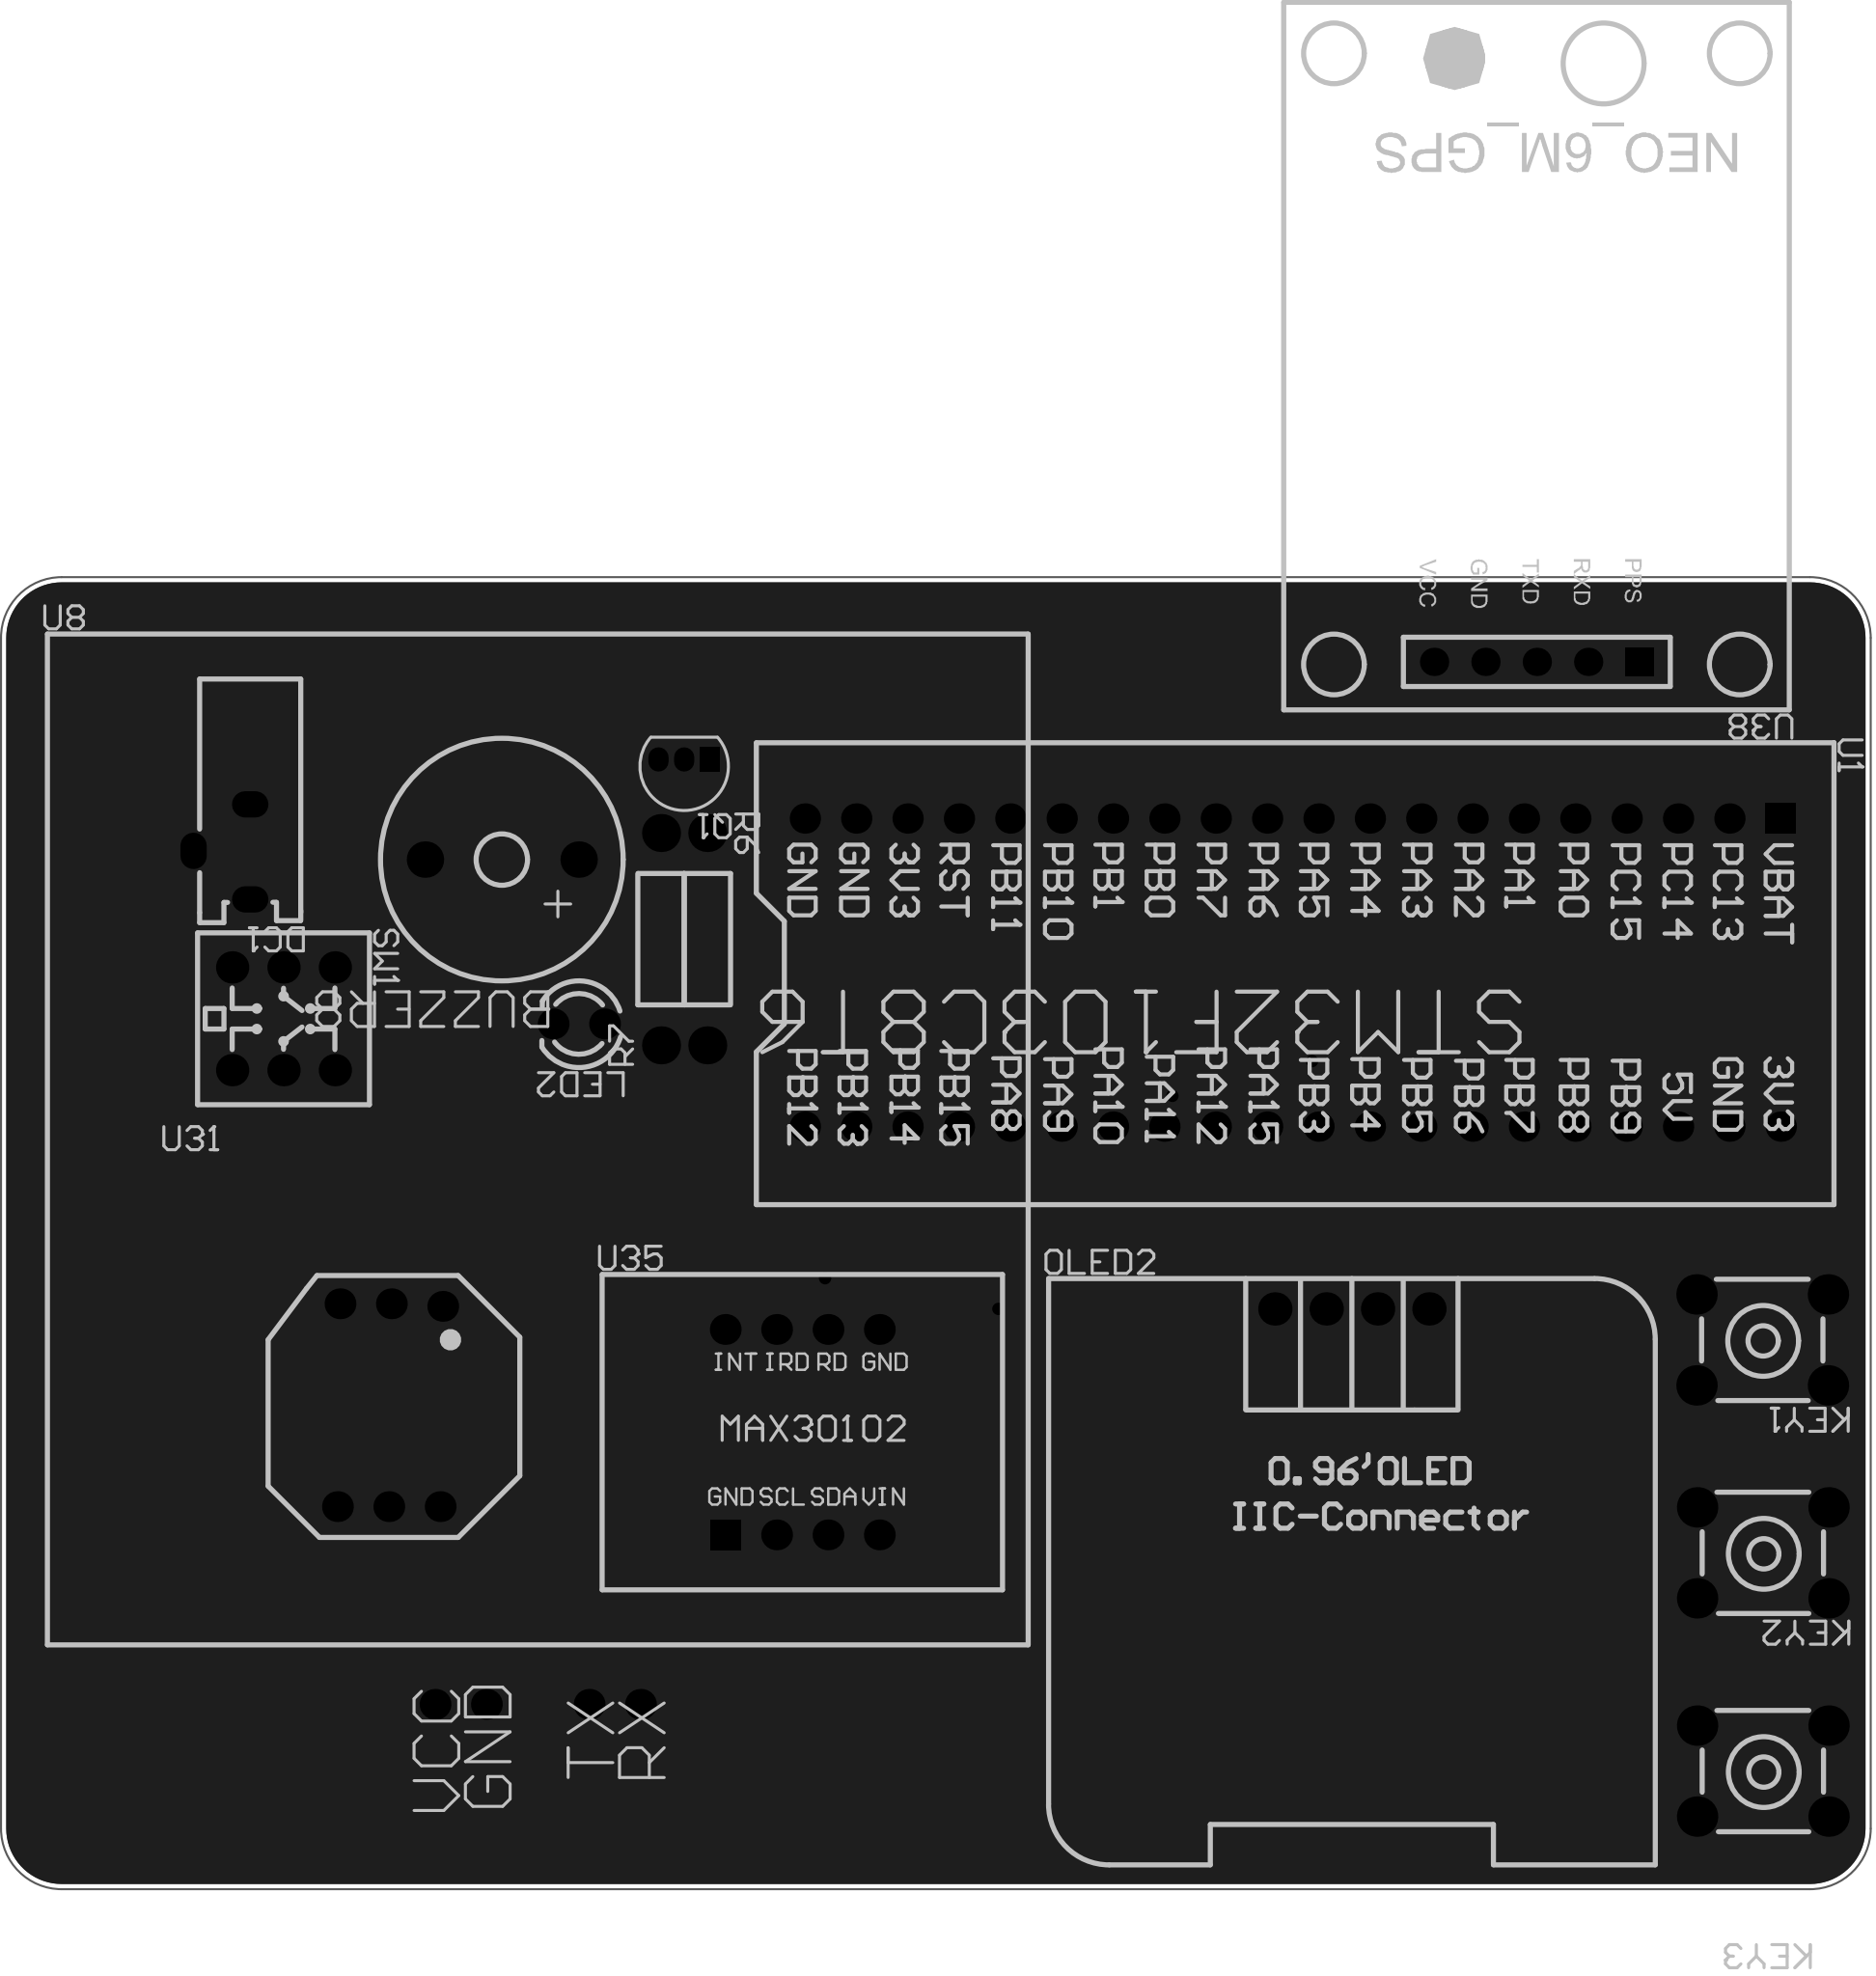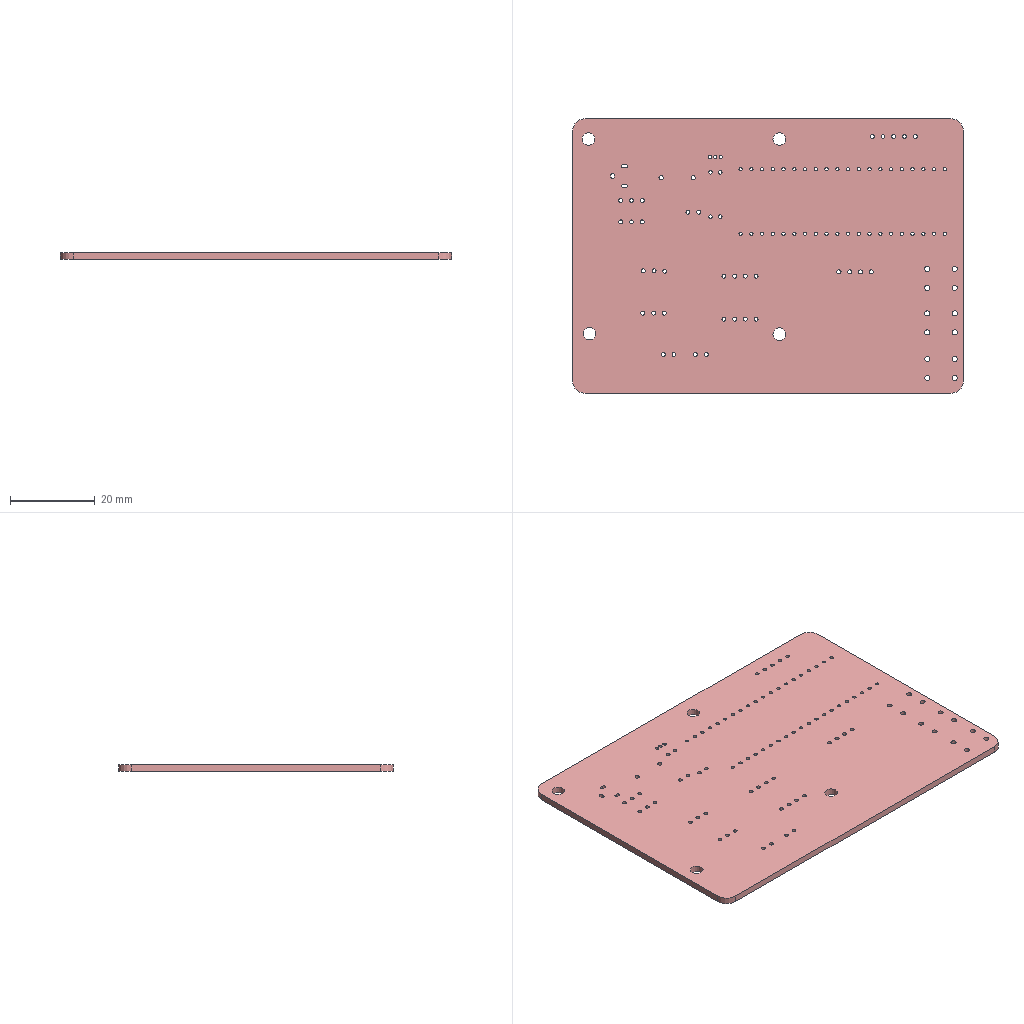Circuit board layout | Altium Designer | box 92.5 x 64.9 x 1.6 mm
Layer stack:
# Altium Designer layer stack of  (unit mm; dielectric type: 0 none, 1 core, 2 prepreg, 3 surface material)
index,name,kind,layer,copper_thickness_mm,dielectric_type,dielectric_thickness_mm,dielectric_material,dielectric_constant
0,Top Paste Mask Layer,other,,,,,,
1,Top Silkscreen Layer,other,,,,,,
2,Top Solder Mask Layer,dielectric,,,3,0.01,,3.3
3,Top Layer,copper,Top Layer,0.035,,,,
4,Dielectric1,dielectric,,,3,1.51,FR4,4.5
5,Bottom Layer,copper,Bottom Layer,0.035,,,,
6,Bottom Solder Mask Layer,dielectric,,,3,0.01,,3.3
7,Bottom Silkscreen Layer,other,,,,,,
8,Bottom Paste Mask Layer,other,,,,,,
# drill layer pairs: low layer,high layer
drill_pair,Top Layer,Bottom Layer
Part placement:
Designator,Comment,Layer,Footprint,Center-X(mm),Center-Y(mm),Rotation
BUZZER8,buzzer-12X9,TopLayer,BUZ-TH_BD12.0-P7.60-D0.6-FD,109.601,153.086,180
DC1,DC002-1.3,TopLayer,DC-IN-TH_DC002-1.3,95.758,153.467,180
KEY1,按键开关6*6*8,TopLayer,KEY-TH_4P-L6.0-W6.0-P4.50-LS7.5,171.929,129.328,180
KEY2,按键开关6*6*8,TopLayer,KEY-TH_4P-L6.0-W6.0-P4.50-LS7.5,171.958,118.796,180
KEY3,按键开关6*6*8,TopLayer,KEY-TH_4P-L6.0-W6.0-P4.50-LS7.5,171.958,108.001,180
LED2,,TopLayer,LED_TH-3mm,113.411,144.958,180
Q1,S8550,TopLayer,TO-92-3_L4.5-W3.5-P1.27-L,118.618,158.039,180
R6,,TopLayer,RES-TH_BD2.3-L6.5-P10.50-D0.5,119.761,149.149,270
R7,,TopLayer,RES-TH_BD2.3-L6.5-P10.50-D0.5,117.475,149.149,90
SW1,,TopLayer,自锁开关8.5*8.5,98.806,145.212,270
U1,STM32F103C8T6-Bluepill,TopLayer,STM32F103C8T6-BLUEPILL,148.717,147.498,270
OLED2,0.96OLED_4P_MODULE_JX,TopLayer,0.96OLED_4P,151.638,130.861,0
U8,SIM900A,TopLayer,SIM900A,111.379,111.303,0
U31,,TopLayer,AGR12_±íÃæÑ¹Á¦´«¸ÐÆ÷,104.076,126.099,0
U35,,TopLayer,MAX30102,124.46,124.765,0
U38,,TopLayer,NEO_6M_GPS模块,160.782,162.865,180
Pad and via stacks:
# Altium Designer via and pad stacks of  (unit mm). Each distinct definition once, with the count of objects using it.
# via: kind,start_layer,end_layer,hole_mm,diameter_mm,mode(0 simple;1 top-mid-bottom;2 full stack),diameter_per_layer,count,example_net
# pad: kind,layer,hole_mm,hole_type(0 round;1 square;2 slot),plating,top_size,top_shape(1 round;2 rect;3 octagon;9 rounded rect),mid_size,bottom_size,mode,footprint,size_per_layer,count,example
pad,Multi-Layer,1.001,0,plated,1.801x1.801,1,1.801x1.801,1.801x1.801,0,BUZ-TH_BD12.0-P7.60-D0.6-FD,,2,BUZZER8.1
pad,Multi-Layer,0.8,2,plated,1.3x1.8,1,1.3x1.8,1.3x1.8,0,DC-IN-TH_DC002-1.3,,3,DC1.1
pad,Multi-Layer,1.2,0,plated,2x2,1,2x2,2x2,0,KEY-TH_4P-L6.0-W6.0-P4.50-LS7.5,,12,KEY1.1
pad,Multi-Layer,0.9144,0,plated,1.524x1.524,1,1.524x1.524,1.524x1.524,0,LED_TH-3mm,,2,LED2.1
pad,Multi-Layer,0.7,2,plated,1x1.2,2,1x1.2,1x1.2,0,TO-92-3_L4.5-W3.5-P1.27-L,,1,Q1.1
pad,Multi-Layer,0.7,2,plated,1x1.2,1,1x1.2,1x1.2,0,TO-92-3_L4.5-W3.5-P1.27-L,,2,Q1.2
pad,Multi-Layer,0.8992,0,plated,1.88x1.88,1,1.88x1.88,1.88x1.88,0,RES-TH_BD2.3-L6.5-P10.50-D0.5,,4,R6.1
pad,Multi-Layer,0.9,0,plated,1.6x1.6,1,1.6x1.6,1.6x1.6,0,\u00D7\u00D4\u00CB\u00F8\u00BF\u00AA\u00B9\u00D88.5*8.5,,6,SW1.1
pad,Multi-Layer,0.8,0,plated,1.5x1.5,1,1.5x1.5,1.5x1.5,0,STM32F103C8T6-BLUEPILL,,39,U1.40
pad,Multi-Layer,0.8,0,plated,1.5x1.5,2,1.5x1.5,1.5x1.5,0,STM32F103C8T6-BLUEPILL,,1,U1.1
pad,Multi-Layer,1,0,plated,1.65x1.65,1,1.65x1.65,1.65x1.65,0,0.96OLED_4P,,4,OLED2.4
pad,Multi-Layer,0.9144,0,plated,1.524x1.524,1,1.524x1.524,1.524x1.524,0,SIM900A,,4,U8.1
pad,Multi-Layer,0.9144,0,plated,1.524x1.524,1,1.524x1.524,1.524x1.524,0,AGR12 \u00B1\u00ED\u00C3\u00E6\u00D1\u00B9\u00C1\u00A6\u00B4\u00AB\u00B8\u00D0\u00C6\u00F7,,6,U31.1
pad,Multi-Layer,0.9144,0,plated,1.524x1.524,1,1.524x1.524,1.524x1.524,0,MAX30102,,7,U35.5
pad,Multi-Layer,0.9144,0,plated,1.524x1.524,2,1.524x1.524,1.524x1.524,0,MAX30102,,1,U35.4
pad,Multi-Layer,0.889,0,plated,1.399x1.399,2,1.399x1.399,1.399x1.399,0,NEO_6M_GPS\u00C4\u00A3\u00BF\u00E9,,1,U38.1
pad,Multi-Layer,0.889,0,plated,1.399x1.399,1,1.399x1.399,1.399x1.399,0,NEO_6M_GPS\u00C4\u00A3\u00BF\u00E9,,4,U38.2
via,Top Layer,Bottom Layer,0.3048,0.61,0,,10,+5V
Copper pours:
name,layer,net,type(0 solid;1 hatched;2 none)
Top Layer-GND,Top Layer,GND,0
Bottom Layer-GND,Bottom Layer,GND,0
Design rules, without the lines most boards share:
# Altium Designer design rules of  (exported by Altium Designer, unit mm)
# columns: name | kind | enabled | priority | scope1 | scope2 | descriptor | typed fields (field=value)
copperThickness1oz_2 | 2 | enabled | 2 | All | All | Width Constraint (Min=5mil) (Max=100mil) (Preferred=19.7mil) (All) |